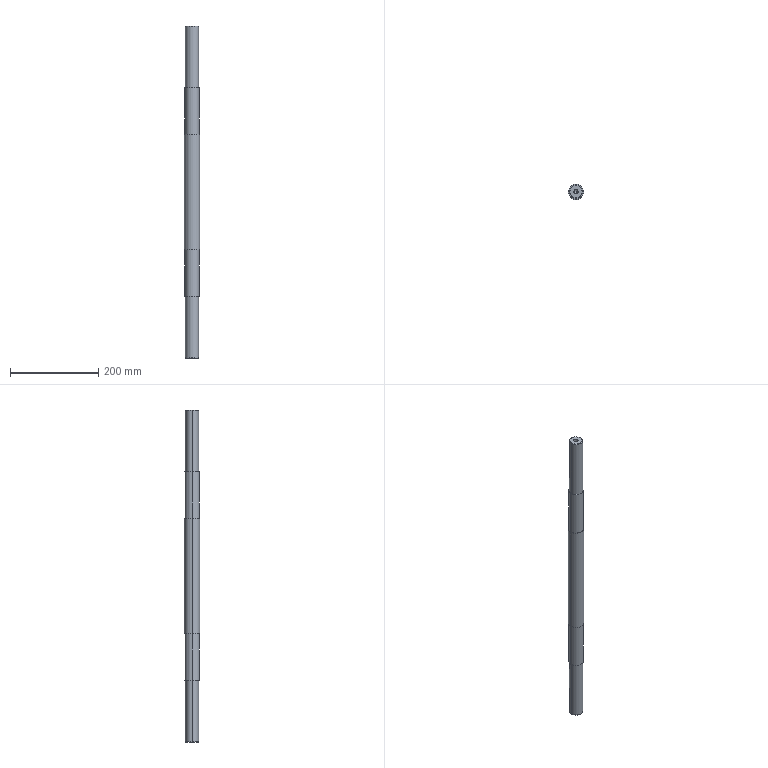Part | STEP file | 1 solid | 28 faces | box 35 x 35 x 753 mm | volume 624999 mm3 | cylinder 14 | cone 8 | plane 6 | commonest cylinder face diameters 10.2 x4 30 x4 33 x4 35 x2